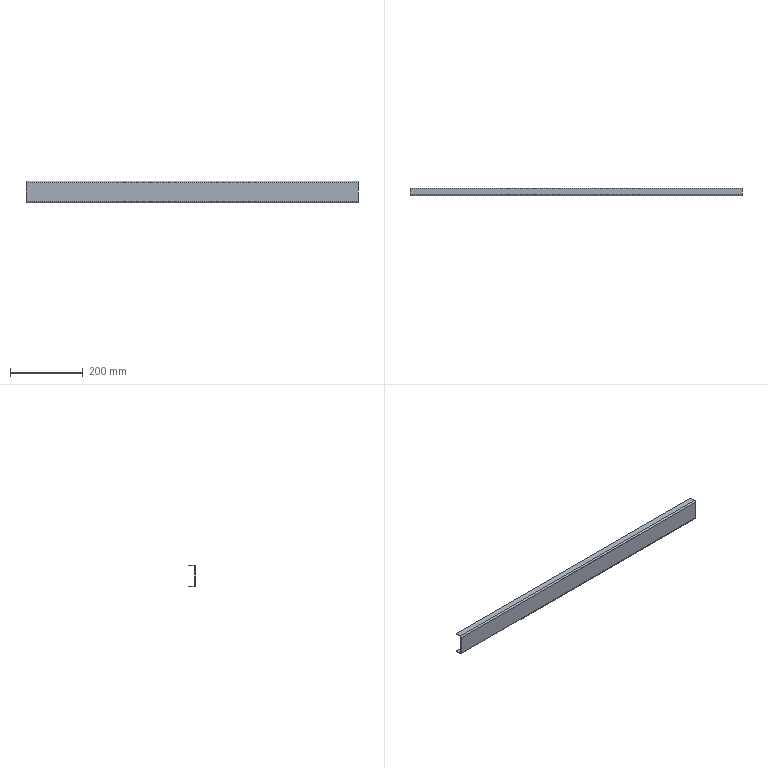Part | NX | features solid 2 | 1 solid | 14 faces | box 910 x 20 x 60 mm | volume 170033 mm3 | plane 10 | cylinder 4 | commonest cylinder face diameters 4 x2 8 x2
STEP:
#1=CARTESIAN_POINT('',(-330.,-18.,710.));
#2=VERTEX_POINT('',#1);
#3=CARTESIAN_POINT('',(-330.,-2.,710.));
#4=VERTEX_POINT('',#3);
#5=CARTESIAN_POINT('',(-330.,-22.,710.));
#6=DIRECTION('',(0.,1.,0.));
#7=VECTOR('',#6,1000.);
#8=LINE('',#5,#7);
#9=EDGE_CURVE('',#2,#4,#8,.T.);
#10=ORIENTED_EDGE('',*,*,#9,.T.);
#11=CARTESIAN_POINT('',(580.,-2.,710.));
#12=VERTEX_POINT('',#11);
#13=CARTESIAN_POINT('',(580.,-2.,710.));
#14=DIRECTION('',(-1.,0.,0.));
#15=VECTOR('',#14,1000.);
#16=LINE('',#13,#15);
#17=EDGE_CURVE('',#12,#4,#16,.T.);
#18=ORIENTED_EDGE('',*,*,#17,.F.);
#19=CARTESIAN_POINT('',(580.,-18.,710.));
#20=VERTEX_POINT('',#19);
#21=CARTESIAN_POINT('',(580.,-22.,710.));
#22=DIRECTION('',(0.,1.,0.));
#23=VECTOR('',#22,1000.);
#24=LINE('',#21,#23);
#25=EDGE_CURVE('',#20,#12,#24,.T.);
#26=ORIENTED_EDGE('',*,*,#25,.F.);
#27=CARTESIAN_POINT('',(580.,-18.,710.));
#28=DIRECTION('',(-1.,0.,0.));
#29=VECTOR('',#28,1000.);
#30=LINE('',#27,#29);
#31=EDGE_CURVE('',#20,#2,#30,.T.);
#32=ORIENTED_EDGE('',*,*,#31,.T.);
#33=EDGE_LOOP('',(#10,#18,#26,#32));
#34=FACE_BOUND('',#33,.T.);
#35=CARTESIAN_POINT('',(580.,-22.,710.));
#36=DIRECTION('',(0.,0.,1.));
#37=DIRECTION('',(0.,-1.,0.));
#38=AXIS2_PLACEMENT_3D('',#35,#36,#37);
#39=PLANE('',#38);
#40=ADVANCED_FACE('',(#34),#39,.F.);
#41=CARTESIAN_POINT('',(-330.,-22.,714.));
#42=VERTEX_POINT('',#41);
#43=CARTESIAN_POINT('',(-330.,-18.,714.));
#44=DIRECTION('',(1.,0.,0.));
#45=DIRECTION('',(0.,1.,0.));
#46=AXIS2_PLACEMENT_3D('',#43,#44,#45);
#47=CIRCLE('',#46,4.);
#48=EDGE_CURVE('',#42,#2,#47,.T.);
#49=ORIENTED_EDGE('',*,*,#48,.T.);
#50=ORIENTED_EDGE('',*,*,#31,.F.);
#51=CARTESIAN_POINT('',(580.,-22.,714.));
#52=VERTEX_POINT('',#51);
#53=CARTESIAN_POINT('',(580.,-18.,714.));
#54=DIRECTION('',(1.,0.,0.));
#55=DIRECTION('',(0.,1.,0.));
#56=AXIS2_PLACEMENT_3D('',#53,#54,#55);
#57=CIRCLE('',#56,4.);
#58=EDGE_CURVE('',#52,#20,#57,.T.);
#59=ORIENTED_EDGE('',*,*,#58,.F.);
#60=CARTESIAN_POINT('',(580.,-22.,714.));
#61=DIRECTION('',(-1.,0.,0.));
#62=VECTOR('',#61,1000.);
#63=LINE('',#60,#62);
#64=EDGE_CURVE('',#52,#42,#63,.T.);
#65=ORIENTED_EDGE('',*,*,#64,.T.);
#66=EDGE_LOOP('',(#49,#50,#59,#65));
#67=FACE_BOUND('',#66,.T.);
#68=CARTESIAN_POINT('',(580.,-18.,714.));
#69=DIRECTION('',(-1.,0.,0.));
#70=DIRECTION('',(0.,1.,0.));
#71=AXIS2_PLACEMENT_3D('',#68,#69,#70);
#72=CYLINDRICAL_SURFACE('',#71,4.);
#73=ADVANCED_FACE('',(#67),#72,.T.);
#74=CARTESIAN_POINT('',(-330.,-22.,766.));
#75=VERTEX_POINT('',#74);
#76=CARTESIAN_POINT('',(-330.,-22.,770.));
#77=DIRECTION('',(0.,0.,-1.));
#78=VECTOR('',#77,1000.);
#79=LINE('',#76,#78);
#80=EDGE_CURVE('',#75,#42,#79,.T.);
#81=ORIENTED_EDGE('',*,*,#80,.T.);
#82=ORIENTED_EDGE('',*,*,#64,.F.);
#83=CARTESIAN_POINT('',(580.,-22.,766.));
#84=VERTEX_POINT('',#83);
#85=CARTESIAN_POINT('',(580.,-22.,770.));
#86=DIRECTION('',(0.,0.,-1.));
#87=VECTOR('',#86,1000.);
#88=LINE('',#85,#87);
#89=EDGE_CURVE('',#84,#52,#88,.T.);
#90=ORIENTED_EDGE('',*,*,#89,.F.);
#91=CARTESIAN_POINT('',(580.,-22.,766.));
#92=DIRECTION('',(-1.,0.,0.));
#93=VECTOR('',#92,1000.);
#94=LINE('',#91,#93);
#95=EDGE_CURVE('',#84,#75,#94,.T.);
#96=ORIENTED_EDGE('',*,*,#95,.T.);
#97=EDGE_LOOP('',(#81,#82,#90,#96));
#98=FACE_BOUND('',#97,.T.);
#99=CARTESIAN_POINT('',(580.,-22.,770.));
#100=DIRECTION('',(0.,1.,0.));
#101=DIRECTION('',(1.,0.,0.));
#102=AXIS2_PLACEMENT_3D('',#99,#100,#101);
#103=PLANE('',#102);
#104=ADVANCED_FACE('',(#98),#103,.F.);
#105=CARTESIAN_POINT('',(-330.,-18.,770.));
#106=VERTEX_POINT('',#105);
#107=CARTESIAN_POINT('',(-330.,-18.,766.));
#108=DIRECTION('',(1.,0.,0.));
#109=DIRECTION('',(0.,1.,0.));
#110=AXIS2_PLACEMENT_3D('',#107,#108,#109);
#111=CIRCLE('',#110,4.);
#112=EDGE_CURVE('',#106,#75,#111,.T.);
#113=ORIENTED_EDGE('',*,*,#112,.T.);
#114=ORIENTED_EDGE('',*,*,#95,.F.);
#115=CARTESIAN_POINT('',(580.,-18.,770.));
#116=VERTEX_POINT('',#115);
#117=CARTESIAN_POINT('',(580.,-18.,766.));
#118=DIRECTION('',(1.,0.,0.));
#119=DIRECTION('',(0.,1.,0.));
#120=AXIS2_PLACEMENT_3D('',#117,#118,#119);
#121=CIRCLE('',#120,4.);
#122=EDGE_CURVE('',#116,#84,#121,.T.);
#123=ORIENTED_EDGE('',*,*,#122,.F.);
#124=CARTESIAN_POINT('',(580.,-18.,770.));
#125=DIRECTION('',(-1.,0.,0.));
#126=VECTOR('',#125,1000.);
#127=LINE('',#124,#126);
#128=EDGE_CURVE('',#116,#106,#127,.T.);
#129=ORIENTED_EDGE('',*,*,#128,.T.);
#130=EDGE_LOOP('',(#113,#114,#123,#129));
#131=FACE_BOUND('',#130,.T.);
#132=CARTESIAN_POINT('',(580.,-18.,766.));
#133=DIRECTION('',(-1.,0.,0.));
#134=DIRECTION('',(0.,1.,0.));
#135=AXIS2_PLACEMENT_3D('',#132,#133,#134);
#136=CYLINDRICAL_SURFACE('',#135,4.);
#137=ADVANCED_FACE('',(#131),#136,.T.);
#138=CARTESIAN_POINT('',(-330.,-2.,770.));
#139=VERTEX_POINT('',#138);
#140=CARTESIAN_POINT('',(-330.,-2.,770.));
#141=DIRECTION('',(0.,-1.,0.));
#142=VECTOR('',#141,1000.);
#143=LINE('',#140,#142);
#144=EDGE_CURVE('',#139,#106,#143,.T.);
#145=ORIENTED_EDGE('',*,*,#144,.T.);
#146=ORIENTED_EDGE('',*,*,#128,.F.);
#147=CARTESIAN_POINT('',(580.,-2.,770.));
#148=VERTEX_POINT('',#147);
#149=CARTESIAN_POINT('',(580.,-2.,770.));
#150=DIRECTION('',(0.,-1.,0.));
#151=VECTOR('',#150,1000.);
#152=LINE('',#149,#151);
#153=EDGE_CURVE('',#148,#116,#152,.T.);
#154=ORIENTED_EDGE('',*,*,#153,.F.);
#155=CARTESIAN_POINT('',(580.,-2.,770.));
#156=DIRECTION('',(-1.,0.,0.));
#157=VECTOR('',#156,1000.);
#158=LINE('',#155,#157);
#159=EDGE_CURVE('',#148,#139,#158,.T.);
#160=ORIENTED_EDGE('',*,*,#159,.T.);
#161=EDGE_LOOP('',(#145,#146,#154,#160));
#162=FACE_BOUND('',#161,.T.);
#163=CARTESIAN_POINT('',(580.,-2.,770.));
#164=DIRECTION('',(0.,0.,-1.));
#165=DIRECTION('',(0.,-1.,0.));
#166=AXIS2_PLACEMENT_3D('',#163,#164,#165);
#167=PLANE('',#166);
#168=ADVANCED_FACE('',(#162),#167,.F.);
#169=CARTESIAN_POINT('',(-330.,-18.,712.));
#170=VERTEX_POINT('',#169);
#171=CARTESIAN_POINT('',(-330.,-2.,712.));
#172=VERTEX_POINT('',#171);
#173=CARTESIAN_POINT('',(-330.,-22.,712.));
#174=DIRECTION('',(0.,1.,0.));
#175=VECTOR('',#174,1000.);
#176=LINE('',#173,#175);
#177=EDGE_CURVE('',#170,#172,#176,.T.);
#178=ORIENTED_EDGE('',*,*,#177,.F.);
#179=CARTESIAN_POINT('',(580.,-18.,712.));
#180=VERTEX_POINT('',#179);
#181=CARTESIAN_POINT('',(580.,-18.,712.));
#182=DIRECTION('',(-1.,0.,0.));
#183=VECTOR('',#182,1000.);
#184=LINE('',#181,#183);
#185=EDGE_CURVE('',#180,#170,#184,.T.);
#186=ORIENTED_EDGE('',*,*,#185,.F.);
#187=CARTESIAN_POINT('',(580.,-2.,712.));
#188=VERTEX_POINT('',#187);
#189=CARTESIAN_POINT('',(580.,-22.,712.));
#190=DIRECTION('',(0.,1.,0.));
#191=VECTOR('',#190,1000.);
#192=LINE('',#189,#191);
#193=EDGE_CURVE('',#180,#188,#192,.T.);
#194=ORIENTED_EDGE('',*,*,#193,.T.);
#195=CARTESIAN_POINT('',(580.,-2.,712.));
#196=DIRECTION('',(-1.,0.,0.));
#197=VECTOR('',#196,1000.);
#198=LINE('',#195,#197);
#199=EDGE_CURVE('',#188,#172,#198,.T.);
#200=ORIENTED_EDGE('',*,*,#199,.T.);
#201=EDGE_LOOP('',(#178,#186,#194,#200));
#202=FACE_BOUND('',#201,.T.);
#203=CARTESIAN_POINT('',(580.,-22.,712.));
#204=DIRECTION('',(0.,0.,1.));
#205=DIRECTION('',(0.,-1.,0.));
#206=AXIS2_PLACEMENT_3D('',#203,#204,#205);
#207=PLANE('',#206);
#208=ADVANCED_FACE('',(#202),#207,.T.);
#209=CARTESIAN_POINT('',(-330.,-20.,714.));
#210=VERTEX_POINT('',#209);
#211=CARTESIAN_POINT('',(-330.,-18.,714.));
#212=DIRECTION('',(1.,0.,0.));
#213=DIRECTION('',(0.,1.,0.));
#214=AXIS2_PLACEMENT_3D('',#211,#212,#213);
#215=CIRCLE('',#214,2.);
#216=EDGE_CURVE('',#210,#170,#215,.T.);
#217=ORIENTED_EDGE('',*,*,#216,.F.);
#218=CARTESIAN_POINT('',(580.,-20.,714.));
#219=VERTEX_POINT('',#218);
#220=CARTESIAN_POINT('',(580.,-20.,714.));
#221=DIRECTION('',(-1.,0.,0.));
#222=VECTOR('',#221,1000.);
#223=LINE('',#220,#222);
#224=EDGE_CURVE('',#219,#210,#223,.T.);
#225=ORIENTED_EDGE('',*,*,#224,.F.);
#226=CARTESIAN_POINT('',(580.,-18.,714.));
#227=DIRECTION('',(1.,0.,0.));
#228=DIRECTION('',(0.,1.,0.));
#229=AXIS2_PLACEMENT_3D('',#226,#227,#228);
#230=CIRCLE('',#229,2.);
#231=EDGE_CURVE('',#219,#180,#230,.T.);
#232=ORIENTED_EDGE('',*,*,#231,.T.);
#233=ORIENTED_EDGE('',*,*,#185,.T.);
#234=EDGE_LOOP('',(#217,#225,#232,#233));
#235=FACE_BOUND('',#234,.T.);
#236=CARTESIAN_POINT('',(580.,-18.,714.));
#237=DIRECTION('',(-1.,0.,0.));
#238=DIRECTION('',(0.,1.,0.));
#239=AXIS2_PLACEMENT_3D('',#236,#237,#238);
#240=CYLINDRICAL_SURFACE('',#239,2.);
#241=ADVANCED_FACE('',(#235),#240,.F.);
#242=CARTESIAN_POINT('',(-330.,-20.,766.));
#243=VERTEX_POINT('',#242);
#244=CARTESIAN_POINT('',(-330.,-20.,770.));
#245=DIRECTION('',(0.,0.,-1.));
#246=VECTOR('',#245,1000.);
#247=LINE('',#244,#246);
#248=EDGE_CURVE('',#243,#210,#247,.T.);
#249=ORIENTED_EDGE('',*,*,#248,.F.);
#250=CARTESIAN_POINT('',(580.,-20.,766.));
#251=VERTEX_POINT('',#250);
#252=CARTESIAN_POINT('',(580.,-20.,766.));
#253=DIRECTION('',(-1.,0.,0.));
#254=VECTOR('',#253,1000.);
#255=LINE('',#252,#254);
#256=EDGE_CURVE('',#251,#243,#255,.T.);
#257=ORIENTED_EDGE('',*,*,#256,.F.);
#258=CARTESIAN_POINT('',(580.,-20.,770.));
#259=DIRECTION('',(0.,0.,-1.));
#260=VECTOR('',#259,1000.);
#261=LINE('',#258,#260);
#262=EDGE_CURVE('',#251,#219,#261,.T.);
#263=ORIENTED_EDGE('',*,*,#262,.T.);
#264=ORIENTED_EDGE('',*,*,#224,.T.);
#265=EDGE_LOOP('',(#249,#257,#263,#264));
#266=FACE_BOUND('',#265,.T.);
#267=CARTESIAN_POINT('',(580.,-20.,770.));
#268=DIRECTION('',(0.,1.,0.));
#269=DIRECTION('',(1.,0.,0.));
#270=AXIS2_PLACEMENT_3D('',#267,#268,#269);
#271=PLANE('',#270);
#272=ADVANCED_FACE('',(#266),#271,.T.);
#273=CARTESIAN_POINT('',(-330.,-18.,768.));
#274=VERTEX_POINT('',#273);
#275=CARTESIAN_POINT('',(-330.,-18.,766.));
#276=DIRECTION('',(1.,0.,0.));
#277=DIRECTION('',(0.,1.,0.));
#278=AXIS2_PLACEMENT_3D('',#275,#276,#277);
#279=CIRCLE('',#278,2.);
#280=EDGE_CURVE('',#274,#243,#279,.T.);
#281=ORIENTED_EDGE('',*,*,#280,.F.);
#282=CARTESIAN_POINT('',(580.,-18.,768.));
#283=VERTEX_POINT('',#282);
#284=CARTESIAN_POINT('',(580.,-18.,768.));
#285=DIRECTION('',(-1.,0.,0.));
#286=VECTOR('',#285,1000.);
#287=LINE('',#284,#286);
#288=EDGE_CURVE('',#283,#274,#287,.T.);
#289=ORIENTED_EDGE('',*,*,#288,.F.);
#290=CARTESIAN_POINT('',(580.,-18.,766.));
#291=DIRECTION('',(1.,0.,0.));
#292=DIRECTION('',(0.,1.,0.));
#293=AXIS2_PLACEMENT_3D('',#290,#291,#292);
#294=CIRCLE('',#293,2.);
#295=EDGE_CURVE('',#283,#251,#294,.T.);
#296=ORIENTED_EDGE('',*,*,#295,.T.);
#297=ORIENTED_EDGE('',*,*,#256,.T.);
#298=EDGE_LOOP('',(#281,#289,#296,#297));
#299=FACE_BOUND('',#298,.T.);
#300=CARTESIAN_POINT('',(580.,-18.,766.));
#301=DIRECTION('',(-1.,0.,0.));
#302=DIRECTION('',(0.,1.,0.));
#303=AXIS2_PLACEMENT_3D('',#300,#301,#302);
#304=CYLINDRICAL_SURFACE('',#303,2.);
#305=ADVANCED_FACE('',(#299),#304,.F.);
#306=CARTESIAN_POINT('',(-330.,-2.,768.));
#307=VERTEX_POINT('',#306);
#308=CARTESIAN_POINT('',(-330.,-2.,768.));
#309=DIRECTION('',(0.,-1.,0.));
#310=VECTOR('',#309,1000.);
#311=LINE('',#308,#310);
#312=EDGE_CURVE('',#307,#274,#311,.T.);
#313=ORIENTED_EDGE('',*,*,#312,.F.);
#314=CARTESIAN_POINT('',(580.,-2.,768.));
#315=VERTEX_POINT('',#314);
#316=CARTESIAN_POINT('',(580.,-2.,768.));
#317=DIRECTION('',(-1.,0.,0.));
#318=VECTOR('',#317,1000.);
#319=LINE('',#316,#318);
#320=EDGE_CURVE('',#315,#307,#319,.T.);
#321=ORIENTED_EDGE('',*,*,#320,.F.);
#322=CARTESIAN_POINT('',(580.,-2.,768.));
#323=DIRECTION('',(0.,-1.,0.));
#324=VECTOR('',#323,1000.);
#325=LINE('',#322,#324);
#326=EDGE_CURVE('',#315,#283,#325,.T.);
#327=ORIENTED_EDGE('',*,*,#326,.T.);
#328=ORIENTED_EDGE('',*,*,#288,.T.);
#329=EDGE_LOOP('',(#313,#321,#327,#328));
#330=FACE_BOUND('',#329,.T.);
#331=CARTESIAN_POINT('',(580.,-2.,768.));
#332=DIRECTION('',(0.,0.,-1.));
#333=DIRECTION('',(0.,-1.,0.));
#334=AXIS2_PLACEMENT_3D('',#331,#332,#333);
#335=PLANE('',#334);
#336=ADVANCED_FACE('',(#330),#335,.T.);
#337=ORIENTED_EDGE('',*,*,#159,.F.);
#338=CARTESIAN_POINT('',(580.,-2.,770.));
#339=DIRECTION('',(0.,0.,-1.));
#340=VECTOR('',#339,1000.);
#341=LINE('',#338,#340);
#342=EDGE_CURVE('',#148,#315,#341,.T.);
#343=ORIENTED_EDGE('',*,*,#342,.T.);
#344=ORIENTED_EDGE('',*,*,#320,.T.);
#345=CARTESIAN_POINT('',(-330.,-2.,770.));
#346=DIRECTION('',(0.,0.,-1.));
#347=VECTOR('',#346,1000.);
#348=LINE('',#345,#347);
#349=EDGE_CURVE('',#139,#307,#348,.T.);
#350=ORIENTED_EDGE('',*,*,#349,.F.);
#351=EDGE_LOOP('',(#337,#343,#344,#350));
#352=FACE_BOUND('',#351,.T.);
#353=CARTESIAN_POINT('',(580.,-2.,770.));
#354=DIRECTION('',(0.,-1.,0.));
#355=DIRECTION('',(0.,0.,-1.));
#356=AXIS2_PLACEMENT_3D('',#353,#354,#355);
#357=PLANE('',#356);
#358=ADVANCED_FACE('',(#352),#357,.F.);
#359=ORIENTED_EDGE('',*,*,#312,.T.);
#360=ORIENTED_EDGE('',*,*,#280,.T.);
#361=ORIENTED_EDGE('',*,*,#248,.T.);
#362=ORIENTED_EDGE('',*,*,#216,.T.);
#363=ORIENTED_EDGE('',*,*,#177,.T.);
#364=CARTESIAN_POINT('',(-330.,-2.,710.));
#365=DIRECTION('',(0.,0.,1.));
#366=VECTOR('',#365,1000.);
#367=LINE('',#364,#366);
#368=EDGE_CURVE('',#4,#172,#367,.T.);
#369=ORIENTED_EDGE('',*,*,#368,.F.);
#370=ORIENTED_EDGE('',*,*,#9,.F.);
#371=ORIENTED_EDGE('',*,*,#48,.F.);
#372=ORIENTED_EDGE('',*,*,#80,.F.);
#373=ORIENTED_EDGE('',*,*,#112,.F.);
#374=ORIENTED_EDGE('',*,*,#144,.F.);
#375=ORIENTED_EDGE('',*,*,#349,.T.);
#376=EDGE_LOOP('',(#359,#360,#361,#362,#363,#369,#370,#371,#372,#373,#374,#375));
#377=FACE_BOUND('',#376,.T.);
#378=CARTESIAN_POINT('',(-330.,-2.,770.));
#379=DIRECTION('',(1.,0.,0.));
#380=DIRECTION('',(0.,1.,0.));
#381=AXIS2_PLACEMENT_3D('',#378,#379,#380);
#382=PLANE('',#381);
#383=ADVANCED_FACE('',(#377),#382,.F.);
#384=CARTESIAN_POINT('',(580.,-2.,710.));
#385=DIRECTION('',(0.,0.,1.));
#386=VECTOR('',#385,1000.);
#387=LINE('',#384,#386);
#388=EDGE_CURVE('',#12,#188,#387,.T.);
#389=ORIENTED_EDGE('',*,*,#388,.F.);
#390=ORIENTED_EDGE('',*,*,#17,.T.);
#391=ORIENTED_EDGE('',*,*,#368,.T.);
#392=ORIENTED_EDGE('',*,*,#199,.F.);
#393=EDGE_LOOP('',(#389,#390,#391,#392));
#394=FACE_BOUND('',#393,.T.);
#395=CARTESIAN_POINT('',(580.,-2.,710.));
#396=DIRECTION('',(0.,1.,0.));
#397=DIRECTION('',(1.,0.,0.));
#398=AXIS2_PLACEMENT_3D('',#395,#396,#397);
#399=PLANE('',#398);
#400=ADVANCED_FACE('',(#394),#399,.T.);
#401=ORIENTED_EDGE('',*,*,#193,.F.);
#402=ORIENTED_EDGE('',*,*,#231,.F.);
#403=ORIENTED_EDGE('',*,*,#262,.F.);
#404=ORIENTED_EDGE('',*,*,#295,.F.);
#405=ORIENTED_EDGE('',*,*,#326,.F.);
#406=ORIENTED_EDGE('',*,*,#342,.F.);
#407=ORIENTED_EDGE('',*,*,#153,.T.);
#408=ORIENTED_EDGE('',*,*,#122,.T.);
#409=ORIENTED_EDGE('',*,*,#89,.T.);
#410=ORIENTED_EDGE('',*,*,#58,.T.);
#411=ORIENTED_EDGE('',*,*,#25,.T.);
#412=ORIENTED_EDGE('',*,*,#388,.T.);
#413=EDGE_LOOP('',(#401,#402,#403,#404,#405,#406,#407,#408,#409,#410,#411,#412));
#414=FACE_BOUND('',#413,.T.);
#415=CARTESIAN_POINT('',(580.,-22.,710.));
#416=DIRECTION('',(1.,0.,0.));
#417=DIRECTION('',(0.,1.,0.));
#418=AXIS2_PLACEMENT_3D('',#415,#416,#417);
#419=PLANE('',#418);
#420=ADVANCED_FACE('',(#414),#419,.T.);
#421=CLOSED_SHELL('',(#40,#73,#104,#137,#168,#208,#241,#272,#305,#336,#358,#383,#400,#420));
#422=MANIFOLD_SOLID_BREP('',#421);
#423=(LENGTH_UNIT()NAMED_UNIT(*)SI_UNIT(.MILLI.,.METRE.));
#424=UNCERTAINTY_MEASURE_WITH_UNIT(LENGTH_MEASURE(0.00001),#423,'','');
#425=(NAMED_UNIT(*)PLANE_ANGLE_UNIT()SI_UNIT($,.RADIAN.));
#426=(NAMED_UNIT(*)SI_UNIT($,.STERADIAN.)SOLID_ANGLE_UNIT());
#427=(GEOMETRIC_REPRESENTATION_CONTEXT(3)GLOBAL_UNCERTAINTY_ASSIGNED_CONTEXT((#424))GLOBAL_UNIT_ASSIGNED_CONTEXT((#423,#425,#426))REPRESENTATION_CONTEXT('',''));
#428=ADVANCED_BREP_SHAPE_REPRESENTATION('',(#422),#427);